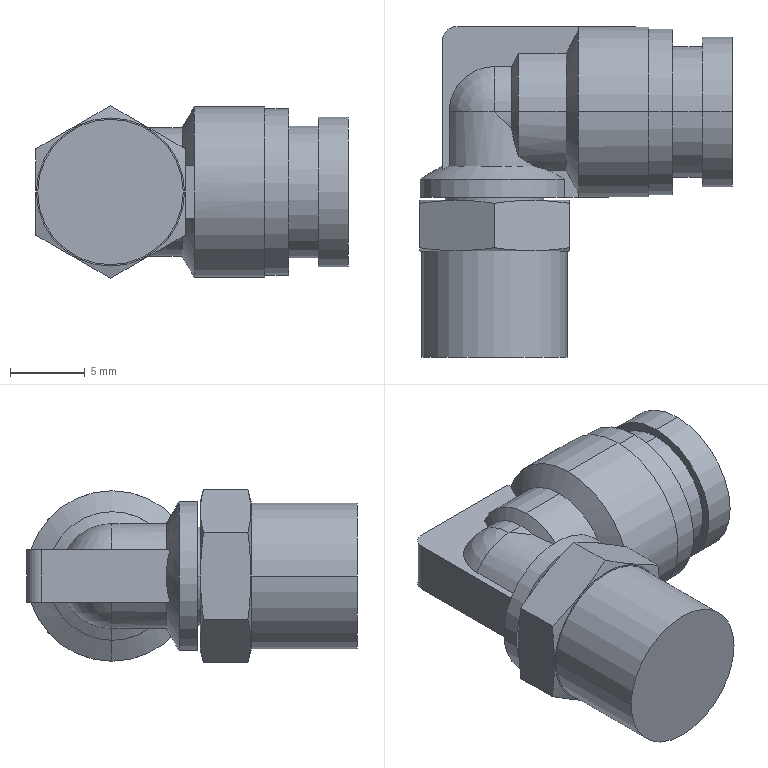Part | SolidWorks | features ICE 2, Revolution 2, HoleWzd 1 | 1 solid | 62 faces | box 20.9 x 22.1 x 11.547 mm | volume 2008 mm3 | plane 25 | cylinder 24 | cone 11 | sphere 2 | commonest cylinder face diameters 7 x5 8.6 x3 10 x3 6 x2 6.6 x2 8.8 x2